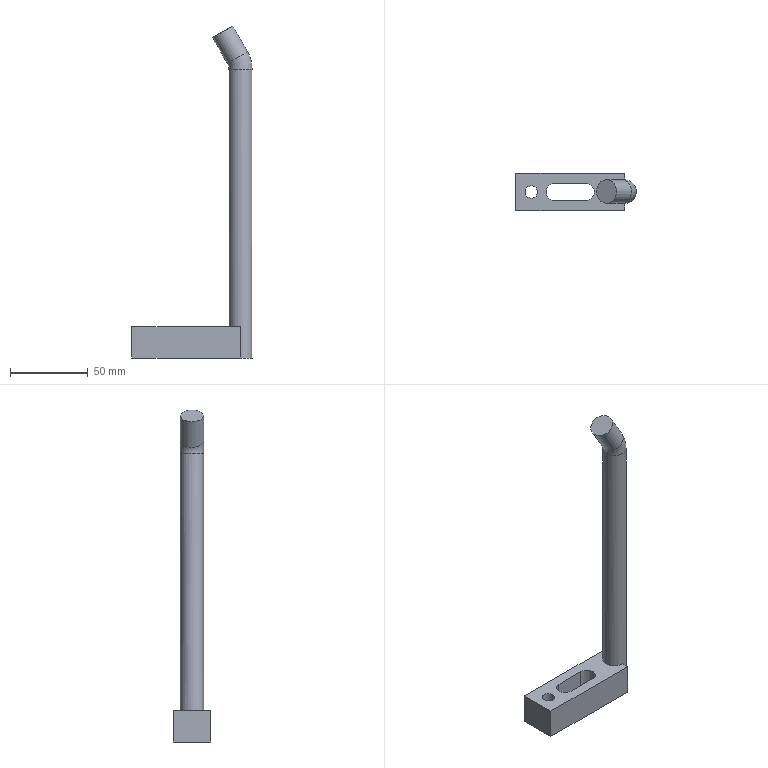Part | NX | features solid 2 | 1 solid | 16 faces | box 77.5 x 24 x 213.75 mm | volume 62151 mm3 | plane 10 | cylinder 5 | torus 1 | commonest cylinder face diameters 11 x2 15 x2 8 x1
STEP:
#1=CARTESIAN_POINT('',(475.5,146.04,30.981));
#2=VERTEX_POINT('',#1);
#3=CARTESIAN_POINT('',(483.,146.04,30.981));
#4=DIRECTION('',(0.,0.,-1.));
#5=DIRECTION('',(-1.,0.,0.));
#6=AXIS2_PLACEMENT_3D('',#3,#4,#5);
#7=CIRCLE('',#6,7.5);
#8=EDGE_CURVE('',#2,#2,#7,.T.);
#9=ORIENTED_EDGE('',*,*,#8,.T.);
#10=EDGE_LOOP('',(#9));
#11=FACE_BOUND('',#10,.T.);
#12=CARTESIAN_POINT('',(483.,138.54,-135.));
#13=VERTEX_POINT('',#12);
#14=CARTESIAN_POINT('',(483.,153.54,-135.));
#15=VERTEX_POINT('',#14);
#16=CARTESIAN_POINT('',(483.,146.04,-135.));
#17=DIRECTION('',(0.,0.,1.));
#18=DIRECTION('',(1.,0.,0.));
#19=AXIS2_PLACEMENT_3D('',#16,#17,#18);
#20=CIRCLE('',#19,7.5);
#21=EDGE_CURVE('',#13,#15,#20,.F.);
#22=ORIENTED_EDGE('',*,*,#21,.F.);
#23=CARTESIAN_POINT('',(483.,138.54,-155.));
#24=VERTEX_POINT('',#23);
#25=CARTESIAN_POINT('',(483.,138.54,-99.019));
#26=DIRECTION('',(0.,0.,-1.));
#27=VECTOR('',#26,1000.);
#28=LINE('',#25,#27);
#29=EDGE_CURVE('',#24,#13,#28,.F.);
#30=ORIENTED_EDGE('',*,*,#29,.F.);
#31=CARTESIAN_POINT('',(483.,153.54,-155.));
#32=VERTEX_POINT('',#31);
#33=CARTESIAN_POINT('',(483.,146.04,-155.));
#34=DIRECTION('',(0.,0.,-1.));
#35=DIRECTION('',(-1.,0.,0.));
#36=AXIS2_PLACEMENT_3D('',#33,#34,#35);
#37=CIRCLE('',#36,7.5);
#38=EDGE_CURVE('',#32,#24,#37,.T.);
#39=ORIENTED_EDGE('',*,*,#38,.F.);
#40=CARTESIAN_POINT('',(483.,153.54,-99.019));
#41=DIRECTION('',(0.,0.,-1.));
#42=VECTOR('',#41,1000.);
#43=LINE('',#40,#42);
#44=EDGE_CURVE('',#15,#32,#43,.T.);
#45=ORIENTED_EDGE('',*,*,#44,.F.);
#46=EDGE_LOOP('',(#22,#30,#39,#45));
#47=FACE_BOUND('',#46,.T.);
#48=CARTESIAN_POINT('',(483.,146.04,-79.019));
#49=DIRECTION('',(0.,0.,-1.));
#50=DIRECTION('',(1.,0.,0.));
#51=AXIS2_PLACEMENT_3D('',#48,#49,#50);
#52=CYLINDRICAL_SURFACE('',#51,7.5);
#53=ADVANCED_FACE('',(#11,#47),#52,.T.);
#54=CARTESIAN_POINT('',(474.495,146.04,34.731));
#55=VERTEX_POINT('',#54);
#56=CARTESIAN_POINT('',(480.99,146.04,38.481));
#57=DIRECTION('',(0.5,0.,-0.866));
#58=DIRECTION('',(-0.866,0.,-0.5));
#59=AXIS2_PLACEMENT_3D('',#56,#57,#58);
#60=CIRCLE('',#59,7.5);
#61=EDGE_CURVE('',#55,#55,#60,.T.);
#62=ORIENTED_EDGE('',*,*,#61,.F.);
#63=EDGE_LOOP('',(#62));
#64=FACE_BOUND('',#63,.T.);
#65=CARTESIAN_POINT('',(464.958,146.04,51.25));
#66=VERTEX_POINT('',#65);
#67=CARTESIAN_POINT('',(471.453,146.04,55.));
#68=DIRECTION('',(0.5,0.,-0.866));
#69=DIRECTION('',(-0.866,0.,-0.5));
#70=AXIS2_PLACEMENT_3D('',#67,#68,#69);
#71=CIRCLE('',#70,7.5);
#72=EDGE_CURVE('',#66,#66,#71,.T.);
#73=ORIENTED_EDGE('',*,*,#72,.T.);
#74=EDGE_LOOP('',(#73));
#75=FACE_BOUND('',#74,.T.);
#76=CARTESIAN_POINT('',(480.99,146.04,38.481));
#77=DIRECTION('',(-0.5,0.,0.866));
#78=DIRECTION('',(-0.866,0.,-0.5));
#79=AXIS2_PLACEMENT_3D('',#76,#77,#78);
#80=CYLINDRICAL_SURFACE('',#79,7.5);
#81=ADVANCED_FACE('',(#64,#75),#80,.T.);
#82=ORIENTED_EDGE('',*,*,#8,.F.);
#83=EDGE_LOOP('',(#82));
#84=FACE_BOUND('',#83,.T.);
#85=ORIENTED_EDGE('',*,*,#61,.T.);
#86=EDGE_LOOP('',(#85));
#87=FACE_BOUND('',#86,.T.);
#88=CARTESIAN_POINT('',(468.,146.04,30.981));
#89=DIRECTION('',(0.,1.,0.));
#90=DIRECTION('',(0.,0.,1.));
#91=AXIS2_PLACEMENT_3D('',#88,#89,#90);
#92=TOROIDAL_SURFACE('',#91,15.,7.5);
#93=ADVANCED_FACE('',(#84,#87),#92,.T.);
#94=ORIENTED_EDGE('',*,*,#72,.F.);
#95=EDGE_LOOP('',(#94));
#96=FACE_BOUND('',#95,.T.);
#97=CARTESIAN_POINT('',(471.453,146.04,55.));
#98=DIRECTION('',(-0.5,0.,0.866));
#99=DIRECTION('',(-0.866,0.,-0.5));
#100=AXIS2_PLACEMENT_3D('',#97,#98,#99);
#101=PLANE('',#100);
#102=ADVANCED_FACE('',(#96),#101,.T.);
#103=CARTESIAN_POINT('',(483.,134.04,-155.));
#104=VERTEX_POINT('',#103);
#105=CARTESIAN_POINT('',(483.,158.04,-155.));
#106=DIRECTION('',(0.,-1.,0.));
#107=VECTOR('',#106,1000.);
#108=LINE('',#105,#107);
#109=EDGE_CURVE('',#24,#104,#108,.T.);
#110=ORIENTED_EDGE('',*,*,#109,.T.);
#111=CARTESIAN_POINT('',(413.,134.04,-155.));
#112=VERTEX_POINT('',#111);
#113=CARTESIAN_POINT('',(483.,134.04,-155.));
#114=DIRECTION('',(-1.,0.,0.));
#115=VECTOR('',#114,1000.);
#116=LINE('',#113,#115);
#117=EDGE_CURVE('',#104,#112,#116,.T.);
#118=ORIENTED_EDGE('',*,*,#117,.T.);
#119=CARTESIAN_POINT('',(413.,158.04,-155.));
#120=VERTEX_POINT('',#119);
#121=CARTESIAN_POINT('',(413.,134.04,-155.));
#122=DIRECTION('',(0.,1.,0.));
#123=VECTOR('',#122,1000.);
#124=LINE('',#121,#123);
#125=EDGE_CURVE('',#112,#120,#124,.T.);
#126=ORIENTED_EDGE('',*,*,#125,.T.);
#127=CARTESIAN_POINT('',(483.,158.04,-155.));
#128=VERTEX_POINT('',#127);
#129=CARTESIAN_POINT('',(413.,158.04,-155.));
#130=DIRECTION('',(1.,0.,0.));
#131=VECTOR('',#130,1000.);
#132=LINE('',#129,#131);
#133=EDGE_CURVE('',#120,#128,#132,.T.);
#134=ORIENTED_EDGE('',*,*,#133,.T.);
#135=CARTESIAN_POINT('',(483.,158.04,-155.));
#136=DIRECTION('',(0.,-1.,0.));
#137=VECTOR('',#136,1000.);
#138=LINE('',#135,#137);
#139=EDGE_CURVE('',#128,#32,#138,.T.);
#140=ORIENTED_EDGE('',*,*,#139,.T.);
#141=ORIENTED_EDGE('',*,*,#38,.T.);
#142=EDGE_LOOP('',(#110,#118,#126,#134,#140,#141));
#143=FACE_BOUND('',#142,.T.);
#144=CARTESIAN_POINT('',(438.,140.54,-155.));
#145=VERTEX_POINT('',#144);
#146=CARTESIAN_POINT('',(438.,151.54,-155.));
#147=VERTEX_POINT('',#146);
#148=CARTESIAN_POINT('',(438.,146.04,-155.));
#149=DIRECTION('',(0.,0.,-1.));
#150=DIRECTION('',(-1.,0.,0.));
#151=AXIS2_PLACEMENT_3D('',#148,#149,#150);
#152=CIRCLE('',#151,5.5);
#153=EDGE_CURVE('',#145,#147,#152,.T.);
#154=ORIENTED_EDGE('',*,*,#153,.F.);
#155=CARTESIAN_POINT('',(458.,140.54,-155.));
#156=VERTEX_POINT('',#155);
#157=CARTESIAN_POINT('',(458.,140.54,-155.));
#158=DIRECTION('',(-1.,0.,0.));
#159=VECTOR('',#158,1000.);
#160=LINE('',#157,#159);
#161=EDGE_CURVE('',#156,#145,#160,.T.);
#162=ORIENTED_EDGE('',*,*,#161,.F.);
#163=CARTESIAN_POINT('',(458.,151.54,-155.));
#164=VERTEX_POINT('',#163);
#165=CARTESIAN_POINT('',(458.,146.04,-155.));
#166=DIRECTION('',(0.,0.,-1.));
#167=DIRECTION('',(-1.,0.,0.));
#168=AXIS2_PLACEMENT_3D('',#165,#166,#167);
#169=CIRCLE('',#168,5.5);
#170=EDGE_CURVE('',#164,#156,#169,.T.);
#171=ORIENTED_EDGE('',*,*,#170,.F.);
#172=CARTESIAN_POINT('',(458.,151.54,-155.));
#173=DIRECTION('',(-1.,0.,0.));
#174=VECTOR('',#173,1000.);
#175=LINE('',#172,#174);
#176=EDGE_CURVE('',#164,#147,#175,.T.);
#177=ORIENTED_EDGE('',*,*,#176,.T.);
#178=EDGE_LOOP('',(#154,#162,#171,#177));
#179=FACE_BOUND('',#178,.T.);
#180=CARTESIAN_POINT('',(419.,146.04,-155.));
#181=VERTEX_POINT('',#180);
#182=CARTESIAN_POINT('',(423.,146.04,-155.));
#183=DIRECTION('',(0.,0.,-1.));
#184=DIRECTION('',(-1.,0.,0.));
#185=AXIS2_PLACEMENT_3D('',#182,#183,#184);
#186=CIRCLE('',#185,4.);
#187=EDGE_CURVE('',#181,#181,#186,.T.);
#188=ORIENTED_EDGE('',*,*,#187,.F.);
#189=EDGE_LOOP('',(#188));
#190=FACE_BOUND('',#189,.T.);
#191=CARTESIAN_POINT('',(413.,158.04,-155.));
#192=DIRECTION('',(0.,0.,1.));
#193=DIRECTION('',(-1.,0.,0.));
#194=AXIS2_PLACEMENT_3D('',#191,#192,#193);
#195=PLANE('',#194);
#196=ADVANCED_FACE('',(#143,#179,#190),#195,.F.);
#197=ORIENTED_EDGE('',*,*,#117,.F.);
#198=CARTESIAN_POINT('',(483.,134.04,-135.));
#199=VERTEX_POINT('',#198);
#200=CARTESIAN_POINT('',(483.,134.04,-135.));
#201=DIRECTION('',(0.,0.,-1.));
#202=VECTOR('',#201,1000.);
#203=LINE('',#200,#202);
#204=EDGE_CURVE('',#199,#104,#203,.T.);
#205=ORIENTED_EDGE('',*,*,#204,.F.);
#206=CARTESIAN_POINT('',(413.,134.04,-135.));
#207=VERTEX_POINT('',#206);
#208=CARTESIAN_POINT('',(483.,134.04,-135.));
#209=DIRECTION('',(-1.,0.,0.));
#210=VECTOR('',#209,1000.);
#211=LINE('',#208,#210);
#212=EDGE_CURVE('',#199,#207,#211,.T.);
#213=ORIENTED_EDGE('',*,*,#212,.T.);
#214=CARTESIAN_POINT('',(413.,134.04,-135.));
#215=DIRECTION('',(0.,0.,-1.));
#216=VECTOR('',#215,1000.);
#217=LINE('',#214,#216);
#218=EDGE_CURVE('',#207,#112,#217,.T.);
#219=ORIENTED_EDGE('',*,*,#218,.T.);
#220=EDGE_LOOP('',(#197,#205,#213,#219));
#221=FACE_BOUND('',#220,.T.);
#222=CARTESIAN_POINT('',(483.,134.04,-135.));
#223=DIRECTION('',(0.,1.,0.));
#224=DIRECTION('',(1.,0.,0.));
#225=AXIS2_PLACEMENT_3D('',#222,#223,#224);
#226=PLANE('',#225);
#227=ADVANCED_FACE('',(#221),#226,.F.);
#228=ORIENTED_EDGE('',*,*,#125,.F.);
#229=ORIENTED_EDGE('',*,*,#218,.F.);
#230=CARTESIAN_POINT('',(413.,158.04,-135.));
#231=VERTEX_POINT('',#230);
#232=CARTESIAN_POINT('',(413.,134.04,-135.));
#233=DIRECTION('',(0.,1.,0.));
#234=VECTOR('',#233,1000.);
#235=LINE('',#232,#234);
#236=EDGE_CURVE('',#207,#231,#235,.T.);
#237=ORIENTED_EDGE('',*,*,#236,.T.);
#238=CARTESIAN_POINT('',(413.,158.04,-135.));
#239=DIRECTION('',(0.,0.,-1.));
#240=VECTOR('',#239,1000.);
#241=LINE('',#238,#240);
#242=EDGE_CURVE('',#231,#120,#241,.T.);
#243=ORIENTED_EDGE('',*,*,#242,.T.);
#244=EDGE_LOOP('',(#228,#229,#237,#243));
#245=FACE_BOUND('',#244,.T.);
#246=CARTESIAN_POINT('',(413.,134.04,-135.));
#247=DIRECTION('',(1.,0.,0.));
#248=DIRECTION('',(0.,0.,1.));
#249=AXIS2_PLACEMENT_3D('',#246,#247,#248);
#250=PLANE('',#249);
#251=ADVANCED_FACE('',(#245),#250,.F.);
#252=ORIENTED_EDGE('',*,*,#133,.F.);
#253=ORIENTED_EDGE('',*,*,#242,.F.);
#254=CARTESIAN_POINT('',(483.,158.04,-135.));
#255=VERTEX_POINT('',#254);
#256=CARTESIAN_POINT('',(413.,158.04,-135.));
#257=DIRECTION('',(1.,0.,0.));
#258=VECTOR('',#257,1000.);
#259=LINE('',#256,#258);
#260=EDGE_CURVE('',#231,#255,#259,.T.);
#261=ORIENTED_EDGE('',*,*,#260,.T.);
#262=CARTESIAN_POINT('',(483.,158.04,-135.));
#263=DIRECTION('',(0.,0.,-1.));
#264=VECTOR('',#263,1000.);
#265=LINE('',#262,#264);
#266=EDGE_CURVE('',#255,#128,#265,.T.);
#267=ORIENTED_EDGE('',*,*,#266,.T.);
#268=EDGE_LOOP('',(#252,#253,#261,#267));
#269=FACE_BOUND('',#268,.T.);
#270=CARTESIAN_POINT('',(413.,158.04,-135.));
#271=DIRECTION('',(0.,-1.,0.));
#272=DIRECTION('',(-1.,0.,0.));
#273=AXIS2_PLACEMENT_3D('',#270,#271,#272);
#274=PLANE('',#273);
#275=ADVANCED_FACE('',(#269),#274,.F.);
#276=ORIENTED_EDGE('',*,*,#44,.T.);
#277=ORIENTED_EDGE('',*,*,#139,.F.);
#278=ORIENTED_EDGE('',*,*,#266,.F.);
#279=CARTESIAN_POINT('',(483.,158.04,-135.));
#280=DIRECTION('',(0.,-1.,0.));
#281=VECTOR('',#280,1000.);
#282=LINE('',#279,#281);
#283=EDGE_CURVE('',#255,#15,#282,.T.);
#284=ORIENTED_EDGE('',*,*,#283,.T.);
#285=EDGE_LOOP('',(#276,#277,#278,#284));
#286=FACE_BOUND('',#285,.T.);
#287=CARTESIAN_POINT('',(483.,158.04,-135.));
#288=DIRECTION('',(-1.,0.,0.));
#289=DIRECTION('',(0.,0.,-1.));
#290=AXIS2_PLACEMENT_3D('',#287,#288,#289);
#291=PLANE('',#290);
#292=ADVANCED_FACE('',(#286),#291,.F.);
#293=ORIENTED_EDGE('',*,*,#29,.T.);
#294=CARTESIAN_POINT('',(483.,158.04,-135.));
#295=DIRECTION('',(0.,-1.,0.));
#296=VECTOR('',#295,1000.);
#297=LINE('',#294,#296);
#298=EDGE_CURVE('',#13,#199,#297,.T.);
#299=ORIENTED_EDGE('',*,*,#298,.T.);
#300=ORIENTED_EDGE('',*,*,#204,.T.);
#301=ORIENTED_EDGE('',*,*,#109,.F.);
#302=EDGE_LOOP('',(#293,#299,#300,#301));
#303=FACE_BOUND('',#302,.T.);
#304=CARTESIAN_POINT('',(483.,158.04,-135.));
#305=DIRECTION('',(-1.,0.,0.));
#306=DIRECTION('',(0.,0.,-1.));
#307=AXIS2_PLACEMENT_3D('',#304,#305,#306);
#308=PLANE('',#307);
#309=ADVANCED_FACE('',(#303),#308,.F.);
#310=CARTESIAN_POINT('',(438.,140.54,-135.));
#311=VERTEX_POINT('',#310);
#312=CARTESIAN_POINT('',(438.,151.54,-135.));
#313=VERTEX_POINT('',#312);
#314=CARTESIAN_POINT('',(438.,146.04,-135.));
#315=DIRECTION('',(0.,0.,-1.));
#316=DIRECTION('',(-1.,0.,0.));
#317=AXIS2_PLACEMENT_3D('',#314,#315,#316);
#318=CIRCLE('',#317,5.5);
#319=EDGE_CURVE('',#311,#313,#318,.T.);
#320=ORIENTED_EDGE('',*,*,#319,.F.);
#321=CARTESIAN_POINT('',(438.,140.54,-135.));
#322=DIRECTION('',(0.,0.,1.));
#323=VECTOR('',#322,1000.);
#324=LINE('',#321,#323);
#325=EDGE_CURVE('',#145,#311,#324,.T.);
#326=ORIENTED_EDGE('',*,*,#325,.F.);
#327=ORIENTED_EDGE('',*,*,#153,.T.);
#328=CARTESIAN_POINT('',(438.,151.54,-135.));
#329=DIRECTION('',(0.,0.,1.));
#330=VECTOR('',#329,1000.);
#331=LINE('',#328,#330);
#332=EDGE_CURVE('',#147,#313,#331,.T.);
#333=ORIENTED_EDGE('',*,*,#332,.T.);
#334=EDGE_LOOP('',(#320,#326,#327,#333));
#335=FACE_BOUND('',#334,.T.);
#336=CARTESIAN_POINT('',(438.,146.04,-135.));
#337=DIRECTION('',(0.,0.,1.));
#338=DIRECTION('',(-1.,0.,0.));
#339=AXIS2_PLACEMENT_3D('',#336,#337,#338);
#340=CYLINDRICAL_SURFACE('',#339,5.5);
#341=ADVANCED_FACE('',(#335),#340,.F.);
#342=CARTESIAN_POINT('',(458.,140.54,-135.));
#343=VERTEX_POINT('',#342);
#344=CARTESIAN_POINT('',(448.,140.54,-135.));
#345=DIRECTION('',(-1.,0.,0.));
#346=VECTOR('',#345,1000.);
#347=LINE('',#344,#346);
#348=EDGE_CURVE('',#343,#311,#347,.T.);
#349=ORIENTED_EDGE('',*,*,#348,.F.);
#350=CARTESIAN_POINT('',(458.,140.54,-135.));
#351=DIRECTION('',(0.,0.,1.));
#352=VECTOR('',#351,1000.);
#353=LINE('',#350,#352);
#354=EDGE_CURVE('',#156,#343,#353,.T.);
#355=ORIENTED_EDGE('',*,*,#354,.F.);
#356=ORIENTED_EDGE('',*,*,#161,.T.);
#357=ORIENTED_EDGE('',*,*,#325,.T.);
#358=EDGE_LOOP('',(#349,#355,#356,#357));
#359=FACE_BOUND('',#358,.T.);
#360=CARTESIAN_POINT('',(448.,140.54,-135.));
#361=DIRECTION('',(0.,-1.,0.));
#362=DIRECTION('',(0.,0.,-1.));
#363=AXIS2_PLACEMENT_3D('',#360,#361,#362);
#364=PLANE('',#363);
#365=ADVANCED_FACE('',(#359),#364,.F.);
#366=CARTESIAN_POINT('',(458.,151.54,-135.));
#367=VERTEX_POINT('',#366);
#368=CARTESIAN_POINT('',(458.,146.04,-135.));
#369=DIRECTION('',(0.,0.,-1.));
#370=DIRECTION('',(-1.,0.,0.));
#371=AXIS2_PLACEMENT_3D('',#368,#369,#370);
#372=CIRCLE('',#371,5.5);
#373=EDGE_CURVE('',#367,#343,#372,.T.);
#374=ORIENTED_EDGE('',*,*,#373,.F.);
#375=CARTESIAN_POINT('',(458.,151.54,-135.));
#376=DIRECTION('',(0.,0.,1.));
#377=VECTOR('',#376,1000.);
#378=LINE('',#375,#377);
#379=EDGE_CURVE('',#164,#367,#378,.T.);
#380=ORIENTED_EDGE('',*,*,#379,.F.);
#381=ORIENTED_EDGE('',*,*,#170,.T.);
#382=ORIENTED_EDGE('',*,*,#354,.T.);
#383=EDGE_LOOP('',(#374,#380,#381,#382));
#384=FACE_BOUND('',#383,.T.);
#385=CARTESIAN_POINT('',(458.,146.04,-135.));
#386=DIRECTION('',(0.,0.,1.));
#387=DIRECTION('',(-1.,0.,0.));
#388=AXIS2_PLACEMENT_3D('',#385,#386,#387);
#389=CYLINDRICAL_SURFACE('',#388,5.5);
#390=ADVANCED_FACE('',(#384),#389,.F.);
#391=CARTESIAN_POINT('',(448.,151.54,-135.));
#392=DIRECTION('',(-1.,0.,0.));
#393=VECTOR('',#392,1000.);
#394=LINE('',#391,#393);
#395=EDGE_CURVE('',#367,#313,#394,.T.);
#396=ORIENTED_EDGE('',*,*,#395,.T.);
#397=ORIENTED_EDGE('',*,*,#332,.F.);
#398=ORIENTED_EDGE('',*,*,#176,.F.);
#399=ORIENTED_EDGE('',*,*,#379,.T.);
#400=EDGE_LOOP('',(#396,#397,#398,#399));
#401=FACE_BOUND('',#400,.T.);
#402=CARTESIAN_POINT('',(448.,151.54,-135.));
#403=DIRECTION('',(0.,1.,0.));
#404=DIRECTION('',(0.,0.,1.));
#405=AXIS2_PLACEMENT_3D('',#402,#403,#404);
#406=PLANE('',#405);
#407=ADVANCED_FACE('',(#401),#406,.F.);
#408=CARTESIAN_POINT('',(427.,146.04,-135.));
#409=VERTEX_POINT('',#408);
#410=CARTESIAN_POINT('',(423.,146.04,-135.));
#411=DIRECTION('',(0.,0.,1.));
#412=DIRECTION('',(1.,0.,0.));
#413=AXIS2_PLACEMENT_3D('',#410,#411,#412);
#414=CIRCLE('',#413,4.);
#415=EDGE_CURVE('',#409,#409,#414,.T.);
#416=ORIENTED_EDGE('',*,*,#415,.T.);
#417=EDGE_LOOP('',(#416));
#418=FACE_BOUND('',#417,.T.);
#419=ORIENTED_EDGE('',*,*,#187,.T.);
#420=EDGE_LOOP('',(#419));
#421=FACE_BOUND('',#420,.T.);
#422=CARTESIAN_POINT('',(423.,146.04,-135.));
#423=DIRECTION('',(0.,0.,-1.));
#424=DIRECTION('',(1.,0.,0.));
#425=AXIS2_PLACEMENT_3D('',#422,#423,#424);
#426=CYLINDRICAL_SURFACE('',#425,4.);
#427=ADVANCED_FACE('',(#418,#421),#426,.F.);
#428=ORIENTED_EDGE('',*,*,#415,.F.);
#429=EDGE_LOOP('',(#428));
#430=FACE_BOUND('',#429,.T.);
#431=ORIENTED_EDGE('',*,*,#395,.F.);
#432=ORIENTED_EDGE('',*,*,#373,.T.);
#433=ORIENTED_EDGE('',*,*,#348,.T.);
#434=ORIENTED_EDGE('',*,*,#319,.T.);
#435=EDGE_LOOP('',(#431,#432,#433,#434));
#436=FACE_BOUND('',#435,.T.);
#437=ORIENTED_EDGE('',*,*,#298,.F.);
#438=ORIENTED_EDGE('',*,*,#21,.T.);
#439=ORIENTED_EDGE('',*,*,#283,.F.);
#440=ORIENTED_EDGE('',*,*,#260,.F.);
#441=ORIENTED_EDGE('',*,*,#236,.F.);
#442=ORIENTED_EDGE('',*,*,#212,.F.);
#443=EDGE_LOOP('',(#437,#438,#439,#440,#441,#442));
#444=FACE_BOUND('',#443,.T.);
#445=CARTESIAN_POINT('',(413.,158.04,-135.));
#446=DIRECTION('',(0.,0.,1.));
#447=DIRECTION('',(-1.,0.,0.));
#448=AXIS2_PLACEMENT_3D('',#445,#446,#447);
#449=PLANE('',#448);
#450=ADVANCED_FACE('',(#430,#436,#444),#449,.T.);
#451=CLOSED_SHELL('',(#53,#81,#93,#102,#196,#227,#251,#275,#292,#309,#341,#365,#390,#407,#427,#450));
#452=MANIFOLD_SOLID_BREP('',#451);
#453=(LENGTH_UNIT()NAMED_UNIT(*)SI_UNIT(.MILLI.,.METRE.));
#454=UNCERTAINTY_MEASURE_WITH_UNIT(LENGTH_MEASURE(0.00001),#453,'','');
#455=(NAMED_UNIT(*)PLANE_ANGLE_UNIT()SI_UNIT($,.RADIAN.));
#456=(NAMED_UNIT(*)SI_UNIT($,.STERADIAN.)SOLID_ANGLE_UNIT());
#457=(GEOMETRIC_REPRESENTATION_CONTEXT(3)GLOBAL_UNCERTAINTY_ASSIGNED_CONTEXT((#454))GLOBAL_UNIT_ASSIGNED_CONTEXT((#453,#455,#456))REPRESENTATION_CONTEXT('',''));
#458=ADVANCED_BREP_SHAPE_REPRESENTATION('',(#452),#457);